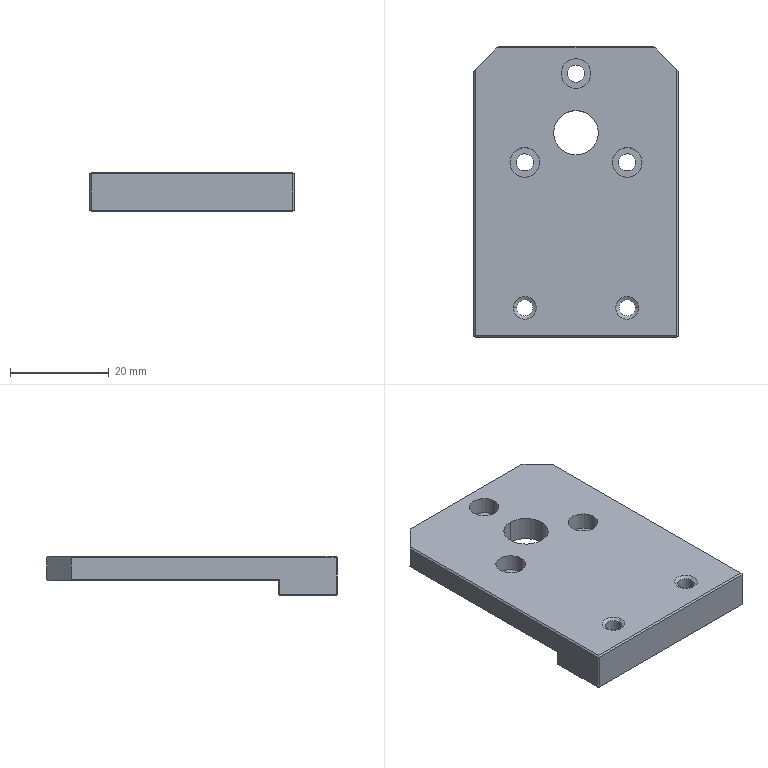Part | NX | 1 solid | 50 faces | box 41.5 x 59 x 8 mm | volume 12794 mm3 | plane 28 | cylinder 18 | cone 4 | commonest cylinder face diameters 3.5 x6 6 x6 3.3 x4 9 x2
STEP:
#1=CARTESIAN_POINT('',(-90.5,196.4,-40.777));
#2=VERTEX_POINT('',#1);
#3=CARTESIAN_POINT('',(-90.5,196.4,-43.777));
#4=VERTEX_POINT('',#3);
#5=CARTESIAN_POINT('',(-90.5,196.4,-42.427));
#6=DIRECTION('',(0.,0.,-1.));
#7=VECTOR('',#6,1000.);
#8=LINE('',#5,#7);
#9=EDGE_CURVE('',#2,#4,#8,.T.);
#10=ORIENTED_EDGE('',*,*,#9,.F.);
#11=CARTESIAN_POINT('',(-90.5,238.7,-40.777));
#12=VERTEX_POINT('',#11);
#13=CARTESIAN_POINT('',(-90.5,217.7,-40.777));
#14=DIRECTION('',(0.,-1.,0.));
#15=VECTOR('',#14,1000.);
#16=LINE('',#13,#15);
#17=EDGE_CURVE('',#12,#2,#16,.T.);
#18=ORIENTED_EDGE('',*,*,#17,.F.);
#19=CARTESIAN_POINT('',(-90.5,238.7,-36.377));
#20=VERTEX_POINT('',#19);
#21=CARTESIAN_POINT('',(-90.5,238.7,-38.577));
#22=DIRECTION('',(0.,0.,-1.));
#23=VECTOR('',#22,1000.);
#24=LINE('',#21,#23);
#25=EDGE_CURVE('',#20,#12,#24,.T.);
#26=ORIENTED_EDGE('',*,*,#25,.F.);
#27=CARTESIAN_POINT('',(-90.5,185.,-36.377));
#28=VERTEX_POINT('',#27);
#29=CARTESIAN_POINT('',(-90.5,211.7,-36.377));
#30=DIRECTION('',(0.,1.,0.));
#31=VECTOR('',#30,1000.);
#32=LINE('',#29,#31);
#33=EDGE_CURVE('',#28,#20,#32,.T.);
#34=ORIENTED_EDGE('',*,*,#33,.F.);
#35=CARTESIAN_POINT('',(-90.5,185.,-43.777));
#36=VERTEX_POINT('',#35);
#37=CARTESIAN_POINT('',(-90.5,185.,-40.077));
#38=DIRECTION('',(0.,0.,-1.));
#39=VECTOR('',#38,1000.);
#40=LINE('',#37,#39);
#41=EDGE_CURVE('',#28,#36,#40,.T.);
#42=ORIENTED_EDGE('',*,*,#41,.T.);
#43=CARTESIAN_POINT('',(-90.5,190.7,-43.777));
#44=DIRECTION('',(0.,-1.,0.));
#45=VECTOR('',#44,1000.);
#46=LINE('',#43,#45);
#47=EDGE_CURVE('',#4,#36,#46,.T.);
#48=ORIENTED_EDGE('',*,*,#47,.F.);
#49=EDGE_LOOP('',(#10,#18,#26,#34,#42,#48));
#50=FACE_BOUND('',#49,.T.);
#51=CARTESIAN_POINT('',(-90.5,208.7,-40.863));
#52=DIRECTION('',(1.,0.,0.));
#53=DIRECTION('',(0.,-1.,0.));
#54=AXIS2_PLACEMENT_3D('',#51,#52,#53);
#55=PLANE('',#54);
#56=ADVANCED_FACE('',(#50),#55,.T.);
#57=CARTESIAN_POINT('',(-131.7,185.,-36.077));
#58=VERTEX_POINT('',#57);
#59=CARTESIAN_POINT('',(-131.7,239.,-36.077));
#60=VERTEX_POINT('',#59);
#61=CARTESIAN_POINT('',(-131.7,0.,-36.077));
#62=DIRECTION('',(0.,1.,0.));
#63=VECTOR('',#62,1000.);
#64=LINE('',#61,#63);
#65=EDGE_CURVE('',#58,#60,#64,.T.);
#66=ORIENTED_EDGE('',*,*,#65,.F.);
#67=CARTESIAN_POINT('',(-90.8,185.,-36.077));
#68=VERTEX_POINT('',#67);
#69=CARTESIAN_POINT('',(0.,185.,-36.077));
#70=DIRECTION('',(1.,0.,0.));
#71=VECTOR('',#70,1000.);
#72=LINE('',#69,#71);
#73=EDGE_CURVE('',#58,#68,#72,.T.);
#74=ORIENTED_EDGE('',*,*,#73,.T.);
#75=CARTESIAN_POINT('',(-90.8,239.,-36.077));
#76=VERTEX_POINT('',#75);
#77=CARTESIAN_POINT('',(-90.8,0.,-36.077));
#78=DIRECTION('',(0.,1.,0.));
#79=VECTOR('',#78,1000.);
#80=LINE('',#77,#79);
#81=EDGE_CURVE('',#68,#76,#80,.T.);
#82=ORIENTED_EDGE('',*,*,#81,.T.);
#83=CARTESIAN_POINT('',(-95.2,243.4,-36.077));
#84=VERTEX_POINT('',#83);
#85=CARTESIAN_POINT('',(148.2,0.,-36.077));
#86=DIRECTION('',(0.7071,-0.7071,0.));
#87=VECTOR('',#86,1000.);
#88=LINE('',#85,#87);
#89=EDGE_CURVE('',#84,#76,#88,.T.);
#90=ORIENTED_EDGE('',*,*,#89,.F.);
#91=CARTESIAN_POINT('',(-127.3,243.4,-36.077));
#92=VERTEX_POINT('',#91);
#93=CARTESIAN_POINT('',(0.,243.4,-36.077));
#94=DIRECTION('',(-1.,0.,0.));
#95=VECTOR('',#94,1000.);
#96=LINE('',#93,#95);
#97=EDGE_CURVE('',#84,#92,#96,.T.);
#98=ORIENTED_EDGE('',*,*,#97,.T.);
#99=CARTESIAN_POINT('',(0.,370.7,-36.077));
#100=DIRECTION('',(0.7071,0.7071,0.));
#101=VECTOR('',#100,1000.);
#102=LINE('',#99,#101);
#103=EDGE_CURVE('',#60,#92,#102,.T.);
#104=ORIENTED_EDGE('',*,*,#103,.F.);
#105=EDGE_LOOP('',(#66,#74,#82,#90,#98,#104));
#106=FACE_BOUND('',#105,.T.);
#107=CARTESIAN_POINT('',(-114.25,238.2,-36.077));
#108=VERTEX_POINT('',#107);
#109=CARTESIAN_POINT('',(-108.25,238.2,-36.077));
#110=VERTEX_POINT('',#109);
#111=CARTESIAN_POINT('',(-111.25,238.2,-36.077));
#112=DIRECTION('',(0.,0.,1.));
#113=DIRECTION('',(-1.,0.,0.));
#114=AXIS2_PLACEMENT_3D('',#111,#112,#113);
#115=CIRCLE('',#114,3.);
#116=EDGE_CURVE('',#108,#110,#115,.T.);
#117=ORIENTED_EDGE('',*,*,#116,.F.);
#118=CARTESIAN_POINT('',(-111.25,238.2,-36.077));
#119=DIRECTION('',(0.,0.,1.));
#120=DIRECTION('',(-1.,0.,0.));
#121=AXIS2_PLACEMENT_3D('',#118,#119,#120);
#122=CIRCLE('',#121,3.);
#123=EDGE_CURVE('',#110,#108,#122,.T.);
#124=ORIENTED_EDGE('',*,*,#123,.F.);
#125=EDGE_LOOP('',(#117,#124));
#126=FACE_BOUND('',#125,.T.);
#127=CARTESIAN_POINT('',(-123.94,190.7,-36.077));
#128=VERTEX_POINT('',#127);
#129=CARTESIAN_POINT('',(-119.31,190.7,-36.077));
#130=VERTEX_POINT('',#129);
#131=CARTESIAN_POINT('',(-121.625,190.7,-36.077));
#132=DIRECTION('',(0.,0.,1.));
#133=DIRECTION('',(1.,0.,0.));
#134=AXIS2_PLACEMENT_3D('',#131,#132,#133);
#135=CIRCLE('',#134,2.315);
#136=EDGE_CURVE('',#128,#130,#135,.T.);
#137=ORIENTED_EDGE('',*,*,#136,.F.);
#138=CARTESIAN_POINT('',(-121.625,190.7,-36.077));
#139=DIRECTION('',(0.,0.,1.));
#140=DIRECTION('',(1.,0.,0.));
#141=AXIS2_PLACEMENT_3D('',#138,#139,#140);
#142=CIRCLE('',#141,2.315);
#143=EDGE_CURVE('',#130,#128,#142,.T.);
#144=ORIENTED_EDGE('',*,*,#143,.F.);
#145=EDGE_LOOP('',(#137,#144));
#146=FACE_BOUND('',#145,.T.);
#147=CARTESIAN_POINT('',(-118.642,220.2,-36.077));
#148=VERTEX_POINT('',#147);
#149=CARTESIAN_POINT('',(-124.642,220.2,-36.077));
#150=VERTEX_POINT('',#149);
#151=CARTESIAN_POINT('',(-121.642,220.2,-36.077));
#152=DIRECTION('',(0.,0.,1.));
#153=DIRECTION('',(-1.,0.,0.));
#154=AXIS2_PLACEMENT_3D('',#151,#152,#153);
#155=CIRCLE('',#154,3.);
#156=EDGE_CURVE('',#148,#150,#155,.T.);
#157=ORIENTED_EDGE('',*,*,#156,.F.);
#158=CARTESIAN_POINT('',(-121.642,220.2,-36.077));
#159=DIRECTION('',(0.,0.,1.));
#160=DIRECTION('',(-1.,0.,0.));
#161=AXIS2_PLACEMENT_3D('',#158,#159,#160);
#162=CIRCLE('',#161,3.);
#163=EDGE_CURVE('',#150,#148,#162,.T.);
#164=ORIENTED_EDGE('',*,*,#163,.F.);
#165=EDGE_LOOP('',(#157,#164));
#166=FACE_BOUND('',#165,.T.);
#167=CARTESIAN_POINT('',(-111.25,230.7,-36.077));
#168=VERTEX_POINT('',#167);
#169=CARTESIAN_POINT('',(-111.25,221.7,-36.077));
#170=VERTEX_POINT('',#169);
#171=CARTESIAN_POINT('',(-111.25,226.2,-36.077));
#172=DIRECTION('',(0.,0.,-1.));
#173=DIRECTION('',(0.,-1.,0.));
#174=AXIS2_PLACEMENT_3D('',#171,#172,#173);
#175=CIRCLE('',#174,4.5);
#176=EDGE_CURVE('',#168,#170,#175,.T.);
#177=ORIENTED_EDGE('',*,*,#176,.T.);
#178=CARTESIAN_POINT('',(-111.25,226.2,-36.077));
#179=DIRECTION('',(0.,0.,-1.));
#180=DIRECTION('',(0.,-1.,0.));
#181=AXIS2_PLACEMENT_3D('',#178,#179,#180);
#182=CIRCLE('',#181,4.5);
#183=EDGE_CURVE('',#170,#168,#182,.T.);
#184=ORIENTED_EDGE('',*,*,#183,.T.);
#185=EDGE_LOOP('',(#177,#184));
#186=FACE_BOUND('',#185,.T.);
#187=CARTESIAN_POINT('',(-97.858,220.2,-36.077));
#188=VERTEX_POINT('',#187);
#189=CARTESIAN_POINT('',(-103.858,220.2,-36.077));
#190=VERTEX_POINT('',#189);
#191=CARTESIAN_POINT('',(-100.858,220.2,-36.077));
#192=DIRECTION('',(0.,0.,1.));
#193=DIRECTION('',(-1.,0.,0.));
#194=AXIS2_PLACEMENT_3D('',#191,#192,#193);
#195=CIRCLE('',#194,3.);
#196=EDGE_CURVE('',#188,#190,#195,.T.);
#197=ORIENTED_EDGE('',*,*,#196,.F.);
#198=CARTESIAN_POINT('',(-100.858,220.2,-36.077));
#199=DIRECTION('',(0.,0.,1.));
#200=DIRECTION('',(-1.,0.,0.));
#201=AXIS2_PLACEMENT_3D('',#198,#199,#200);
#202=CIRCLE('',#201,3.);
#203=EDGE_CURVE('',#190,#188,#202,.T.);
#204=ORIENTED_EDGE('',*,*,#203,.F.);
#205=EDGE_LOOP('',(#197,#204));
#206=FACE_BOUND('',#205,.T.);
#207=CARTESIAN_POINT('',(-103.19,190.7,-36.077));
#208=VERTEX_POINT('',#207);
#209=CARTESIAN_POINT('',(-98.56,190.7,-36.077));
#210=VERTEX_POINT('',#209);
#211=CARTESIAN_POINT('',(-100.875,190.7,-36.077));
#212=DIRECTION('',(0.,0.,1.));
#213=DIRECTION('',(1.,0.,0.));
#214=AXIS2_PLACEMENT_3D('',#211,#212,#213);
#215=CIRCLE('',#214,2.315);
#216=EDGE_CURVE('',#208,#210,#215,.T.);
#217=ORIENTED_EDGE('',*,*,#216,.F.);
#218=CARTESIAN_POINT('',(-100.875,190.7,-36.077));
#219=DIRECTION('',(0.,0.,1.));
#220=DIRECTION('',(1.,0.,0.));
#221=AXIS2_PLACEMENT_3D('',#218,#219,#220);
#222=CIRCLE('',#221,2.315);
#223=EDGE_CURVE('',#210,#208,#222,.T.);
#224=ORIENTED_EDGE('',*,*,#223,.F.);
#225=EDGE_LOOP('',(#217,#224));
#226=FACE_BOUND('',#225,.T.);
#227=CARTESIAN_POINT('',(-137.,208.7,-36.077));
#228=DIRECTION('',(0.,0.,1.));
#229=DIRECTION('',(1.,0.,0.));
#230=AXIS2_PLACEMENT_3D('',#227,#228,#229);
#231=PLANE('',#230);
#232=ADVANCED_FACE('',(#106,#126,#146,#166,#186,#206,#226),#231,.T.);
#233=CARTESIAN_POINT('',(-132.,196.4,-43.777));
#234=VERTEX_POINT('',#233);
#235=CARTESIAN_POINT('',(-132.,196.4,-40.777));
#236=VERTEX_POINT('',#235);
#237=CARTESIAN_POINT('',(-132.,196.4,-42.427));
#238=DIRECTION('',(0.,0.,1.));
#239=VECTOR('',#238,1000.);
#240=LINE('',#237,#239);
#241=EDGE_CURVE('',#234,#236,#240,.T.);
#242=ORIENTED_EDGE('',*,*,#241,.F.);
#243=CARTESIAN_POINT('',(-132.,185.,-43.777));
#244=VERTEX_POINT('',#243);
#245=CARTESIAN_POINT('',(-132.,190.7,-43.777));
#246=DIRECTION('',(0.,1.,0.));
#247=VECTOR('',#246,1000.);
#248=LINE('',#245,#247);
#249=EDGE_CURVE('',#244,#234,#248,.T.);
#250=ORIENTED_EDGE('',*,*,#249,.F.);
#251=CARTESIAN_POINT('',(-132.,185.,-36.377));
#252=VERTEX_POINT('',#251);
#253=CARTESIAN_POINT('',(-132.,185.,-40.077));
#254=DIRECTION('',(0.,0.,1.));
#255=VECTOR('',#254,1000.);
#256=LINE('',#253,#255);
#257=EDGE_CURVE('',#244,#252,#256,.T.);
#258=ORIENTED_EDGE('',*,*,#257,.T.);
#259=CARTESIAN_POINT('',(-132.,238.7,-36.377));
#260=VERTEX_POINT('',#259);
#261=CARTESIAN_POINT('',(-132.,211.7,-36.377));
#262=DIRECTION('',(0.,-1.,0.));
#263=VECTOR('',#262,1000.);
#264=LINE('',#261,#263);
#265=EDGE_CURVE('',#260,#252,#264,.T.);
#266=ORIENTED_EDGE('',*,*,#265,.F.);
#267=CARTESIAN_POINT('',(-132.,238.7,-40.777));
#268=VERTEX_POINT('',#267);
#269=CARTESIAN_POINT('',(-132.,238.7,-38.577));
#270=DIRECTION('',(0.,0.,1.));
#271=VECTOR('',#270,1000.);
#272=LINE('',#269,#271);
#273=EDGE_CURVE('',#268,#260,#272,.T.);
#274=ORIENTED_EDGE('',*,*,#273,.F.);
#275=CARTESIAN_POINT('',(-132.,217.7,-40.777));
#276=DIRECTION('',(0.,1.,0.));
#277=VECTOR('',#276,1000.);
#278=LINE('',#275,#277);
#279=EDGE_CURVE('',#236,#268,#278,.T.);
#280=ORIENTED_EDGE('',*,*,#279,.F.);
#281=EDGE_LOOP('',(#242,#250,#258,#266,#274,#280));
#282=FACE_BOUND('',#281,.T.);
#283=CARTESIAN_POINT('',(-132.,208.7,-44.077));
#284=DIRECTION('',(-1.,0.,0.));
#285=DIRECTION('',(0.,0.,1.));
#286=AXIS2_PLACEMENT_3D('',#283,#284,#285);
#287=PLANE('',#286);
#288=ADVANCED_FACE('',(#282),#287,.T.);
#289=CARTESIAN_POINT('',(-127.3,243.4,-41.077));
#290=VERTEX_POINT('',#289);
#291=CARTESIAN_POINT('',(-95.2,243.4,-41.077));
#292=VERTEX_POINT('',#291);
#293=CARTESIAN_POINT('',(-111.25,243.4,-41.077));
#294=DIRECTION('',(1.,0.,0.));
#295=VECTOR('',#294,1000.);
#296=LINE('',#293,#295);
#297=EDGE_CURVE('',#290,#292,#296,.T.);
#298=ORIENTED_EDGE('',*,*,#297,.T.);
#299=CARTESIAN_POINT('',(-90.8,239.,-41.077));
#300=VERTEX_POINT('',#299);
#301=CARTESIAN_POINT('',(-60.5,208.7,-41.077));
#302=DIRECTION('',(-0.7071,0.7071,0.));
#303=VECTOR('',#302,1000.);
#304=LINE('',#301,#303);
#305=EDGE_CURVE('',#300,#292,#304,.T.);
#306=ORIENTED_EDGE('',*,*,#305,.F.);
#307=CARTESIAN_POINT('',(-90.8,196.7,-41.077));
#308=VERTEX_POINT('',#307);
#309=CARTESIAN_POINT('',(-90.8,217.7,-41.077));
#310=DIRECTION('',(0.,-1.,0.));
#311=VECTOR('',#310,1000.);
#312=LINE('',#309,#311);
#313=EDGE_CURVE('',#300,#308,#312,.T.);
#314=ORIENTED_EDGE('',*,*,#313,.T.);
#315=CARTESIAN_POINT('',(-131.7,196.7,-41.077));
#316=VERTEX_POINT('',#315);
#317=CARTESIAN_POINT('',(-128.319,196.7,-41.077));
#318=DIRECTION('',(1.,0.,0.));
#319=VECTOR('',#318,1000.);
#320=LINE('',#317,#319);
#321=EDGE_CURVE('',#316,#308,#320,.T.);
#322=ORIENTED_EDGE('',*,*,#321,.F.);
#323=CARTESIAN_POINT('',(-131.7,239.,-41.077));
#324=VERTEX_POINT('',#323);
#325=CARTESIAN_POINT('',(-131.7,217.7,-41.077));
#326=DIRECTION('',(0.,1.,0.));
#327=VECTOR('',#326,1000.);
#328=LINE('',#325,#327);
#329=EDGE_CURVE('',#316,#324,#328,.T.);
#330=ORIENTED_EDGE('',*,*,#329,.T.);
#331=CARTESIAN_POINT('',(-162.,208.7,-41.077));
#332=DIRECTION('',(-0.7071,-0.7071,0.));
#333=VECTOR('',#332,1000.);
#334=LINE('',#331,#333);
#335=EDGE_CURVE('',#290,#324,#334,.T.);
#336=ORIENTED_EDGE('',*,*,#335,.F.);
#337=EDGE_LOOP('',(#298,#306,#314,#322,#330,#336));
#338=FACE_BOUND('',#337,.T.);
#339=CARTESIAN_POINT('',(-111.25,230.7,-41.077));
#340=VERTEX_POINT('',#339);
#341=CARTESIAN_POINT('',(-111.25,221.7,-41.077));
#342=VERTEX_POINT('',#341);
#343=CARTESIAN_POINT('',(-111.25,226.2,-41.077));
#344=DIRECTION('',(0.,0.,-1.));
#345=DIRECTION('',(0.,-1.,0.));
#346=AXIS2_PLACEMENT_3D('',#343,#344,#345);
#347=CIRCLE('',#346,4.5);
#348=EDGE_CURVE('',#340,#342,#347,.T.);
#349=ORIENTED_EDGE('',*,*,#348,.F.);
#350=CARTESIAN_POINT('',(-111.25,226.2,-41.077));
#351=DIRECTION('',(0.,0.,-1.));
#352=DIRECTION('',(0.,-1.,0.));
#353=AXIS2_PLACEMENT_3D('',#350,#351,#352);
#354=CIRCLE('',#353,4.5);
#355=EDGE_CURVE('',#342,#340,#354,.T.);
#356=ORIENTED_EDGE('',*,*,#355,.F.);
#357=EDGE_LOOP('',(#349,#356));
#358=FACE_BOUND('',#357,.T.);
#359=CARTESIAN_POINT('',(-123.392,220.2,-41.077));
#360=VERTEX_POINT('',#359);
#361=CARTESIAN_POINT('',(-119.892,220.2,-41.077));
#362=VERTEX_POINT('',#361);
#363=CARTESIAN_POINT('',(-121.642,220.2,-41.077));
#364=DIRECTION('',(0.,0.,1.));
#365=DIRECTION('',(-1.,0.,0.));
#366=AXIS2_PLACEMENT_3D('',#363,#364,#365);
#367=CIRCLE('',#366,1.75);
#368=EDGE_CURVE('',#360,#362,#367,.T.);
#369=ORIENTED_EDGE('',*,*,#368,.T.);
#370=CARTESIAN_POINT('',(-121.642,220.2,-41.077));
#371=DIRECTION('',(0.,0.,1.));
#372=DIRECTION('',(-1.,0.,0.));
#373=AXIS2_PLACEMENT_3D('',#370,#371,#372);
#374=CIRCLE('',#373,1.75);
#375=EDGE_CURVE('',#362,#360,#374,.T.);
#376=ORIENTED_EDGE('',*,*,#375,.T.);
#377=EDGE_LOOP('',(#369,#376));
#378=FACE_BOUND('',#377,.T.);
#379=CARTESIAN_POINT('',(-113.,238.2,-41.077));
#380=VERTEX_POINT('',#379);
#381=CARTESIAN_POINT('',(-109.5,238.2,-41.077));
#382=VERTEX_POINT('',#381);
#383=CARTESIAN_POINT('',(-111.25,238.2,-41.077));
#384=DIRECTION('',(0.,0.,1.));
#385=DIRECTION('',(-1.,0.,0.));
#386=AXIS2_PLACEMENT_3D('',#383,#384,#385);
#387=CIRCLE('',#386,1.75);
#388=EDGE_CURVE('',#380,#382,#387,.T.);
#389=ORIENTED_EDGE('',*,*,#388,.T.);
#390=CARTESIAN_POINT('',(-111.25,238.2,-41.077));
#391=DIRECTION('',(0.,0.,1.));
#392=DIRECTION('',(-1.,0.,0.));
#393=AXIS2_PLACEMENT_3D('',#390,#391,#392);
#394=CIRCLE('',#393,1.75);
#395=EDGE_CURVE('',#382,#380,#394,.T.);
#396=ORIENTED_EDGE('',*,*,#395,.T.);
#397=EDGE_LOOP('',(#389,#396));
#398=FACE_BOUND('',#397,.T.);
#399=CARTESIAN_POINT('',(-99.108,220.2,-41.077));
#400=VERTEX_POINT('',#399);
#401=CARTESIAN_POINT('',(-102.608,220.2,-41.077));
#402=VERTEX_POINT('',#401);
#403=CARTESIAN_POINT('',(-100.858,220.2,-41.077));
#404=DIRECTION('',(0.,0.,1.));
#405=DIRECTION('',(-1.,0.,0.));
#406=AXIS2_PLACEMENT_3D('',#403,#404,#405);
#407=CIRCLE('',#406,1.75);
#408=EDGE_CURVE('',#400,#402,#407,.T.);
#409=ORIENTED_EDGE('',*,*,#408,.T.);
#410=CARTESIAN_POINT('',(-100.858,220.2,-41.077));
#411=DIRECTION('',(0.,0.,1.));
#412=DIRECTION('',(-1.,0.,0.));
#413=AXIS2_PLACEMENT_3D('',#410,#411,#412);
#414=CIRCLE('',#413,1.75);
#415=EDGE_CURVE('',#402,#400,#414,.T.);
#416=ORIENTED_EDGE('',*,*,#415,.T.);
#417=EDGE_LOOP('',(#409,#416));
#418=FACE_BOUND('',#417,.T.);
#419=CARTESIAN_POINT('',(-122.,208.7,-41.077));
#420=DIRECTION('',(0.,0.,-1.));
#421=DIRECTION('',(0.,-1.,0.));
#422=AXIS2_PLACEMENT_3D('',#419,#420,#421);
#423=PLANE('',#422);
#424=ADVANCED_FACE('',(#338,#358,#378,#398,#418),#423,.T.);
#425=ORIENTED_EDGE('',*,*,#321,.T.);
#426=CARTESIAN_POINT('',(-90.8,196.7,-43.777));
#427=VERTEX_POINT('',#426);
#428=CARTESIAN_POINT('',(-90.8,196.7,-42.427));
#429=DIRECTION('',(0.,0.,-1.));
#430=VECTOR('',#429,1000.);
#431=LINE('',#428,#430);
#432=EDGE_CURVE('',#308,#427,#431,.T.);
#433=ORIENTED_EDGE('',*,*,#432,.T.);
#434=CARTESIAN_POINT('',(-131.7,196.7,-43.777));
#435=VERTEX_POINT('',#434);
#436=CARTESIAN_POINT('',(-111.25,196.7,-43.777));
#437=DIRECTION('',(-1.,0.,0.));
#438=VECTOR('',#437,1000.);
#439=LINE('',#436,#438);
#440=EDGE_CURVE('',#427,#435,#439,.T.);
#441=ORIENTED_EDGE('',*,*,#440,.T.);
#442=CARTESIAN_POINT('',(-131.7,196.7,-42.427));
#443=DIRECTION('',(0.,0.,1.));
#444=VECTOR('',#443,1000.);
#445=LINE('',#442,#444);
#446=EDGE_CURVE('',#435,#316,#445,.T.);
#447=ORIENTED_EDGE('',*,*,#446,.T.);
#448=EDGE_LOOP('',(#425,#433,#441,#447));
#449=FACE_BOUND('',#448,.T.);
#450=CARTESIAN_POINT('',(-85.5,196.7,-41.077));
#451=DIRECTION('',(0.,1.,0.));
#452=DIRECTION('',(1.,0.,0.));
#453=AXIS2_PLACEMENT_3D('',#450,#451,#452);
#454=PLANE('',#453);
#455=ADVANCED_FACE('',(#449),#454,.T.);
#456=CARTESIAN_POINT('',(-90.8,185.,-44.077));
#457=VERTEX_POINT('',#456);
#458=CARTESIAN_POINT('',(-90.8,196.4,-44.077));
#459=VERTEX_POINT('',#458);
#460=CARTESIAN_POINT('',(-90.8,0.,-44.077));
#461=DIRECTION('',(0.,1.,0.));
#462=VECTOR('',#461,1000.);
#463=LINE('',#460,#462);
#464=EDGE_CURVE('',#457,#459,#463,.T.);
#465=ORIENTED_EDGE('',*,*,#464,.F.);
#466=CARTESIAN_POINT('',(-131.7,185.,-44.077));
#467=VERTEX_POINT('',#466);
#468=CARTESIAN_POINT('',(0.,185.,-44.077));
#469=DIRECTION('',(-1.,0.,0.));
#470=VECTOR('',#469,1000.);
#471=LINE('',#468,#470);
#472=EDGE_CURVE('',#457,#467,#471,.T.);
#473=ORIENTED_EDGE('',*,*,#472,.T.);
#474=CARTESIAN_POINT('',(-131.7,196.4,-44.077));
#475=VERTEX_POINT('',#474);
#476=CARTESIAN_POINT('',(-131.7,0.,-44.077));
#477=DIRECTION('',(0.,-1.,0.));
#478=VECTOR('',#477,1000.);
#479=LINE('',#476,#478);
#480=EDGE_CURVE('',#475,#467,#479,.T.);
#481=ORIENTED_EDGE('',*,*,#480,.F.);
#482=CARTESIAN_POINT('',(0.,196.4,-44.077));
#483=DIRECTION('',(1.,0.,0.));
#484=VECTOR('',#483,1000.);
#485=LINE('',#482,#484);
#486=EDGE_CURVE('',#475,#459,#485,.T.);
#487=ORIENTED_EDGE('',*,*,#486,.T.);
#488=EDGE_LOOP('',(#465,#473,#481,#487));
#489=FACE_BOUND('',#488,.T.);
#490=CARTESIAN_POINT('',(-102.525,190.7,-44.077));
#491=VERTEX_POINT('',#490);
#492=CARTESIAN_POINT('',(-99.225,190.7,-44.077));
#493=VERTEX_POINT('',#492);
#494=CARTESIAN_POINT('',(-100.875,190.7,-44.077));
#495=DIRECTION('',(0.,0.,1.));
#496=DIRECTION('',(1.,0.,0.));
#497=AXIS2_PLACEMENT_3D('',#494,#495,#496);
#498=CIRCLE('',#497,1.65);
#499=EDGE_CURVE('',#491,#493,#498,.T.);
#500=ORIENTED_EDGE('',*,*,#499,.T.);
#501=CARTESIAN_POINT('',(-100.875,190.7,-44.077));
#502=DIRECTION('',(0.,0.,1.));
#503=DIRECTION('',(1.,0.,0.));
#504=AXIS2_PLACEMENT_3D('',#501,#502,#503);
#505=CIRCLE('',#504,1.65);
#506=EDGE_CURVE('',#493,#491,#505,.T.);
#507=ORIENTED_EDGE('',*,*,#506,.T.);
#508=EDGE_LOOP('',(#500,#507));
#509=FACE_BOUND('',#508,.T.);
#510=CARTESIAN_POINT('',(-123.275,190.7,-44.077));
#511=VERTEX_POINT('',#510);
#512=CARTESIAN_POINT('',(-119.975,190.7,-44.077));
#513=VERTEX_POINT('',#512);
#514=CARTESIAN_POINT('',(-121.625,190.7,-44.077));
#515=DIRECTION('',(0.,0.,1.));
#516=DIRECTION('',(1.,0.,0.));
#517=AXIS2_PLACEMENT_3D('',#514,#515,#516);
#518=CIRCLE('',#517,1.65);
#519=EDGE_CURVE('',#511,#513,#518,.T.);
#520=ORIENTED_EDGE('',*,*,#519,.T.);
#521=CARTESIAN_POINT('',(-121.625,190.7,-44.077));
#522=DIRECTION('',(0.,0.,1.));
#523=DIRECTION('',(1.,0.,0.));
#524=AXIS2_PLACEMENT_3D('',#521,#522,#523);
#525=CIRCLE('',#524,1.65);
#526=EDGE_CURVE('',#513,#511,#525,.T.);
#527=ORIENTED_EDGE('',*,*,#526,.T.);
#528=EDGE_LOOP('',(#520,#527));
#529=FACE_BOUND('',#528,.T.);
#530=CARTESIAN_POINT('',(-88.698,210.445,-44.077));
#531=DIRECTION('',(0.,0.,-1.));
#532=DIRECTION('',(0.,-1.,0.));
#533=AXIS2_PLACEMENT_3D('',#530,#531,#532);
#534=PLANE('',#533);
#535=ADVANCED_FACE('',(#489,#509,#529),#534,.T.);
#536=ORIENTED_EDGE('',*,*,#348,.T.);
#537=CARTESIAN_POINT('',(-111.25,221.7,-35.277));
#538=DIRECTION('',(0.,0.,-1.));
#539=VECTOR('',#538,1000.);
#540=LINE('',#537,#539);
#541=EDGE_CURVE('',#342,#170,#540,.F.);
#542=ORIENTED_EDGE('',*,*,#541,.T.);
#543=ORIENTED_EDGE('',*,*,#176,.F.);
#544=CARTESIAN_POINT('',(-111.25,230.7,-35.277));
#545=DIRECTION('',(0.,0.,-1.));
#546=VECTOR('',#545,1000.);
#547=LINE('',#544,#546);
#548=EDGE_CURVE('',#340,#168,#547,.F.);
#549=ORIENTED_EDGE('',*,*,#548,.F.);
#550=EDGE_LOOP('',(#536,#542,#543,#549));
#551=FACE_BOUND('',#550,.T.);
#552=CARTESIAN_POINT('',(-111.25,226.2,-35.277));
#553=DIRECTION('',(0.,0.,-1.));
#554=DIRECTION('',(0.,-1.,0.));
#555=AXIS2_PLACEMENT_3D('',#552,#553,#554);
#556=CYLINDRICAL_SURFACE('',#555,4.5);
#557=ADVANCED_FACE('',(#551),#556,.F.);
#558=ORIENTED_EDGE('',*,*,#464,.T.);
#559=CARTESIAN_POINT('',(-90.65,196.55,-43.927));
#560=VERTEX_POINT('',#559);
#561=CARTESIAN_POINT('',(-78.5,208.7,-31.777));
#562=DIRECTION('',(0.5774,0.5774,0.5774));
#563=VECTOR('',#562,1000.);
#564=LINE('',#561,#563);
#565=EDGE_CURVE('',#459,#560,#564,.T.);
#566=ORIENTED_EDGE('',*,*,#565,.T.);
#567=CARTESIAN_POINT('',(-89.502,195.402,-42.779));
#568=DIRECTION('',(0.5774,-0.5774,0.5774));
#569=VECTOR('',#568,1000.);
#570=LINE('',#567,#569);
#571=EDGE_CURVE('',#560,#4,#570,.T.);
#572=ORIENTED_EDGE('',*,*,#571,.T.);
#573=ORIENTED_EDGE('',*,*,#47,.T.);
#574=CARTESIAN_POINT('',(-90.65,184.85,-43.927));
#575=VERTEX_POINT('',#574);
#576=CARTESIAN_POINT('',(-66.8,208.7,-20.077));
#577=DIRECTION('',(0.5774,0.5774,0.5774));
#578=VECTOR('',#577,1000.);
#579=LINE('',#576,#578);
#580=EDGE_CURVE('',#575,#36,#579,.T.);
#581=ORIENTED_EDGE('',*,*,#580,.F.);
#582=CARTESIAN_POINT('',(-114.5,208.7,-67.777));
#583=DIRECTION('',(-0.5774,0.5774,-0.5774));
#584=VECTOR('',#583,1000.);
#585=LINE('',#582,#584);
#586=EDGE_CURVE('',#575,#457,#585,.T.);
#587=ORIENTED_EDGE('',*,*,#586,.T.);
#588=EDGE_LOOP('',(#558,#566,#572,#573,#581,#587));
#589=FACE_BOUND('',#588,.T.);
#590=CARTESIAN_POINT('',(-90.65,190.7,-43.927));
#591=DIRECTION('',(0.7071,0.,-0.7071));
#592=DIRECTION('',(0.,-1.,0.));
#593=AXIS2_PLACEMENT_3D('',#590,#591,#592);
#594=PLANE('',#593);
#595=ADVANCED_FACE('',(#589),#594,.T.);
#596=ORIENTED_EDGE('',*,*,#33,.T.);
#597=CARTESIAN_POINT('',(-84.098,232.298,-42.779));
#598=DIRECTION('',(0.5774,-0.5774,-0.5774));
#599=VECTOR('',#598,1000.);
#600=LINE('',#597,#599);
#601=EDGE_CURVE('',#76,#20,#600,.T.);
#602=ORIENTED_EDGE('',*,*,#601,.F.);
#603=ORIENTED_EDGE('',*,*,#81,.F.);
#604=CARTESIAN_POINT('',(-90.65,184.85,-36.227));
#605=VERTEX_POINT('',#604);
#606=CARTESIAN_POINT('',(-114.5,208.7,-12.377));
#607=DIRECTION('',(-0.5774,0.5774,0.5774));
#608=VECTOR('',#607,1000.);
#609=LINE('',#606,#608);
#610=EDGE_CURVE('',#605,#68,#609,.T.);
#611=ORIENTED_EDGE('',*,*,#610,.F.);
#612=CARTESIAN_POINT('',(-66.8,208.7,-60.077));
#613=DIRECTION('',(0.5774,0.5774,-0.5774));
#614=VECTOR('',#613,1000.);
#615=LINE('',#612,#614);
#616=EDGE_CURVE('',#605,#28,#615,.T.);
#617=ORIENTED_EDGE('',*,*,#616,.T.);
#618=EDGE_LOOP('',(#596,#602,#603,#611,#617));
#619=FACE_BOUND('',#618,.T.);
#620=CARTESIAN_POINT('',(-90.65,211.7,-36.227));
#621=DIRECTION('',(-0.7071,0.,-0.7071));
#622=DIRECTION('',(-0.7071,0.,0.7071));
#623=AXIS2_PLACEMENT_3D('',#620,#621,#622);
#624=PLANE('',#623);
#625=ADVANCED_FACE('',(#619),#624,.F.);
#626=ORIENTED_EDGE('',*,*,#472,.F.);
#627=ORIENTED_EDGE('',*,*,#586,.F.);
#628=CARTESIAN_POINT('',(-90.8,184.7,-43.777));
#629=VERTEX_POINT('',#628);
#630=CARTESIAN_POINT('',(-66.8,208.7,-67.777));
#631=DIRECTION('',(-0.5774,-0.5774,0.5774));
#632=VECTOR('',#631,1000.);
#633=LINE('',#630,#632);
#634=EDGE_CURVE('',#575,#629,#633,.T.);
#635=ORIENTED_EDGE('',*,*,#634,.T.);
#636=CARTESIAN_POINT('',(-131.7,184.7,-43.777));
#637=VERTEX_POINT('',#636);
#638=CARTESIAN_POINT('',(-111.25,184.7,-43.777));
#639=DIRECTION('',(1.,0.,0.));
#640=VECTOR('',#639,1000.);
#641=LINE('',#638,#640);
#642=EDGE_CURVE('',#637,#629,#641,.T.);
#643=ORIENTED_EDGE('',*,*,#642,.F.);
#644=CARTESIAN_POINT('',(-131.85,184.85,-43.927));
#645=VERTEX_POINT('',#644);
#646=CARTESIAN_POINT('',(-155.7,208.7,-67.777));
#647=DIRECTION('',(0.5774,-0.5774,0.5774));
#648=VECTOR('',#647,1000.);
#649=LINE('',#646,#648);
#650=EDGE_CURVE('',#645,#637,#649,.T.);
#651=ORIENTED_EDGE('',*,*,#650,.F.);
#652=CARTESIAN_POINT('',(-108.,208.7,-67.777));
#653=DIRECTION('',(0.5774,0.5774,-0.5774));
#654=VECTOR('',#653,1000.);
#655=LINE('',#652,#654);
#656=EDGE_CURVE('',#645,#467,#655,.T.);
#657=ORIENTED_EDGE('',*,*,#656,.T.);
#658=EDGE_LOOP('',(#626,#627,#635,#643,#651,#657));
#659=FACE_BOUND('',#658,.T.);
#660=CARTESIAN_POINT('',(-111.25,184.85,-43.927));
#661=DIRECTION('',(0.,0.7071,0.7071));
#662=DIRECTION('',(1.,0.,0.));
#663=AXIS2_PLACEMENT_3D('',#660,#661,#662);
#664=PLANE('',#663);
#665=ADVANCED_FACE('',(#659),#664,.F.);
#666=ORIENTED_EDGE('',*,*,#486,.F.);
#667=CARTESIAN_POINT('',(-131.85,196.55,-43.927));
#668=VERTEX_POINT('',#667);
#669=CARTESIAN_POINT('',(-132.998,197.698,-42.779));
#670=DIRECTION('',(-0.5774,0.5774,0.5774));
#671=VECTOR('',#670,1000.);
#672=LINE('',#669,#671);
#673=EDGE_CURVE('',#475,#668,#672,.T.);
#674=ORIENTED_EDGE('',*,*,#673,.T.);
#675=CARTESIAN_POINT('',(-119.7,208.7,-31.777));
#676=DIRECTION('',(-0.5774,-0.5774,-0.5774));
#677=VECTOR('',#676,1000.);
#678=LINE('',#675,#677);
#679=EDGE_CURVE('',#435,#668,#678,.T.);
#680=ORIENTED_EDGE('',*,*,#679,.F.);
#681=ORIENTED_EDGE('',*,*,#440,.F.);
#682=CARTESIAN_POINT('',(-91.798,197.698,-42.779));
#683=DIRECTION('',(-0.5774,0.5774,0.5774));
#684=VECTOR('',#683,1000.);
#685=LINE('',#682,#684);
#686=EDGE_CURVE('',#560,#427,#685,.T.);
#687=ORIENTED_EDGE('',*,*,#686,.F.);
#688=ORIENTED_EDGE('',*,*,#565,.F.);
#689=EDGE_LOOP('',(#666,#674,#680,#681,#687,#688));
#690=FACE_BOUND('',#689,.T.);
#691=CARTESIAN_POINT('',(-111.25,196.55,-43.927));
#692=DIRECTION('',(0.,-0.7071,0.7071));
#693=DIRECTION('',(-1.,0.,0.));
#694=AXIS2_PLACEMENT_3D('',#691,#692,#693);
#695=PLANE('',#694);
#696=ADVANCED_FACE('',(#690),#695,.F.);
#697=ORIENTED_EDGE('',*,*,#9,.T.);
#698=ORIENTED_EDGE('',*,*,#571,.F.);
#699=ORIENTED_EDGE('',*,*,#686,.T.);
#700=ORIENTED_EDGE('',*,*,#432,.F.);
#701=CARTESIAN_POINT('',(-92.502,198.402,-42.779));
#702=DIRECTION('',(0.5774,-0.5774,0.5774));
#703=VECTOR('',#702,1000.);
#704=LINE('',#701,#703);
#705=EDGE_CURVE('',#308,#2,#704,.T.);
#706=ORIENTED_EDGE('',*,*,#705,.T.);
#707=EDGE_LOOP('',(#697,#698,#699,#700,#706));
#708=FACE_BOUND('',#707,.T.);
#709=CARTESIAN_POINT('',(-90.65,196.55,-42.427));
#710=DIRECTION('',(-0.7071,-0.7071,0.));
#711=DIRECTION('',(-0.7071,0.7071,0.));
#712=AXIS2_PLACEMENT_3D('',#709,#710,#711);
#713=PLANE('',#712);
#714=ADVANCED_FACE('',(#708),#713,.F.);
#715=ORIENTED_EDGE('',*,*,#17,.T.);
#716=ORIENTED_EDGE('',*,*,#705,.F.);
#717=ORIENTED_EDGE('',*,*,#313,.F.);
#718=CARTESIAN_POINT('',(-92.502,240.702,-42.779));
#719=DIRECTION('',(-0.5774,0.5774,-0.5774));
#720=VECTOR('',#719,1000.);
#721=LINE('',#718,#720);
#722=EDGE_CURVE('',#12,#300,#721,.T.);
#723=ORIENTED_EDGE('',*,*,#722,.F.);
#724=EDGE_LOOP('',(#715,#716,#717,#723));
#725=FACE_BOUND('',#724,.T.);
#726=CARTESIAN_POINT('',(-90.65,217.7,-40.927));
#727=DIRECTION('',(-0.7071,0.,0.7071));
#728=DIRECTION('',(0.,1.,0.));
#729=AXIS2_PLACEMENT_3D('',#726,#727,#728);
#730=PLANE('',#729);
#731=ADVANCED_FACE('',(#725),#730,.F.);
#732=ORIENTED_EDGE('',*,*,#279,.T.);
#733=CARTESIAN_POINT('',(-162.,208.7,-10.777));
#734=DIRECTION('',(-0.5774,-0.5774,0.5774));
#735=VECTOR('',#734,1000.);
#736=LINE('',#733,#735);
#737=EDGE_CURVE('',#324,#268,#736,.T.);
#738=ORIENTED_EDGE('',*,*,#737,.F.);
#739=ORIENTED_EDGE('',*,*,#329,.F.);
#740=CARTESIAN_POINT('',(-119.7,208.7,-53.077));
#741=DIRECTION('',(0.5774,0.5774,-0.5774));
#742=VECTOR('',#741,1000.);
#743=LINE('',#740,#742);
#744=EDGE_CURVE('',#236,#316,#743,.T.);
#745=ORIENTED_EDGE('',*,*,#744,.F.);
#746=EDGE_LOOP('',(#732,#738,#739,#745));
#747=FACE_BOUND('',#746,.T.);
#748=CARTESIAN_POINT('',(-131.85,217.7,-40.927));
#749=DIRECTION('',(0.7071,0.,0.7071));
#750=DIRECTION('',(0.,-1.,0.));
#751=AXIS2_PLACEMENT_3D('',#748,#749,#750);
#752=PLANE('',#751);
#753=ADVANCED_FACE('',(#747),#752,.F.);
#754=ORIENTED_EDGE('',*,*,#241,.T.);
#755=ORIENTED_EDGE('',*,*,#744,.T.);
#756=ORIENTED_EDGE('',*,*,#446,.F.);
#757=ORIENTED_EDGE('',*,*,#679,.T.);
#758=CARTESIAN_POINT('',(-119.7,208.7,-56.077));
#759=DIRECTION('',(0.5774,0.5774,-0.5774));
#760=VECTOR('',#759,1000.);
#761=LINE('',#758,#760);
#762=EDGE_CURVE('',#234,#668,#761,.T.);
#763=ORIENTED_EDGE('',*,*,#762,.F.);
#764=EDGE_LOOP('',(#754,#755,#756,#757,#763));
#765=FACE_BOUND('',#764,.T.);
#766=CARTESIAN_POINT('',(-131.85,196.55,-42.427));
#767=DIRECTION('',(0.7071,-0.7071,0.));
#768=DIRECTION('',(0.,0.,-1.));
#769=AXIS2_PLACEMENT_3D('',#766,#767,#768);
#770=PLANE('',#769);
#771=ADVANCED_FACE('',(#765),#770,.F.);
#772=CARTESIAN_POINT('',(-95.5,243.7,-36.377));
#773=VERTEX_POINT('',#772);
#774=CARTESIAN_POINT('',(-95.5,243.7,-40.777));
#775=VERTEX_POINT('',#774);
#776=CARTESIAN_POINT('',(-95.5,243.7,-38.577));
#777=DIRECTION('',(0.,0.,-1.));
#778=VECTOR('',#777,1000.);
#779=LINE('',#776,#778);
#780=EDGE_CURVE('',#773,#775,#779,.T.);
#781=ORIENTED_EDGE('',*,*,#780,.F.);
#782=CARTESIAN_POINT('',(-101.902,250.102,-42.779));
#783=DIRECTION('',(0.5774,-0.5774,0.5774));
#784=VECTOR('',#783,1000.);
#785=LINE('',#782,#784);
#786=EDGE_CURVE('',#773,#84,#785,.T.);
#787=ORIENTED_EDGE('',*,*,#786,.T.);
#788=ORIENTED_EDGE('',*,*,#89,.T.);
#789=ORIENTED_EDGE('',*,*,#601,.T.);
#790=ORIENTED_EDGE('',*,*,#25,.T.);
#791=ORIENTED_EDGE('',*,*,#722,.T.);
#792=ORIENTED_EDGE('',*,*,#305,.T.);
#793=CARTESIAN_POINT('',(-93.498,241.698,-42.779));
#794=DIRECTION('',(-0.5774,0.5774,0.5774));
#795=VECTOR('',#794,1000.);
#796=LINE('',#793,#795);
#797=EDGE_CURVE('',#292,#775,#796,.T.);
#798=ORIENTED_EDGE('',*,*,#797,.T.);
#799=EDGE_LOOP('',(#781,#787,#788,#789,#790,#791,#792,#798));
#800=FACE_BOUND('',#799,.T.);
#801=CARTESIAN_POINT('',(-93.,241.2,-38.577));
#802=DIRECTION('',(0.7071,0.7071,0.));
#803=DIRECTION('',(0.,0.,-1.));
#804=AXIS2_PLACEMENT_3D('',#801,#802,#803);
#805=PLANE('',#804);
#806=ADVANCED_FACE('',(#800),#805,.T.);
#807=CARTESIAN_POINT('',(-131.7,184.7,-36.377));
#808=VERTEX_POINT('',#807);
#809=CARTESIAN_POINT('',(-90.8,184.7,-36.377));
#810=VERTEX_POINT('',#809);
#811=CARTESIAN_POINT('',(-111.25,184.7,-36.377));
#812=DIRECTION('',(1.,0.,0.));
#813=VECTOR('',#812,1000.);
#814=LINE('',#811,#813);
#815=EDGE_CURVE('',#808,#810,#814,.T.);
#816=ORIENTED_EDGE('',*,*,#815,.T.);
#817=CARTESIAN_POINT('',(-66.8,208.7,-12.377));
#818=DIRECTION('',(0.5774,0.5774,0.5774));
#819=VECTOR('',#818,1000.);
#820=LINE('',#817,#819);
#821=EDGE_CURVE('',#810,#605,#820,.T.);
#822=ORIENTED_EDGE('',*,*,#821,.T.);
#823=ORIENTED_EDGE('',*,*,#610,.T.);
#824=ORIENTED_EDGE('',*,*,#73,.F.);
#825=CARTESIAN_POINT('',(-131.85,184.85,-36.227));
#826=VERTEX_POINT('',#825);
#827=CARTESIAN_POINT('',(-108.,208.7,-12.377));
#828=DIRECTION('',(0.5774,0.5774,0.5774));
#829=VECTOR('',#828,1000.);
#830=LINE('',#827,#829);
#831=EDGE_CURVE('',#826,#58,#830,.T.);
#832=ORIENTED_EDGE('',*,*,#831,.F.);
#833=CARTESIAN_POINT('',(-155.7,208.7,-12.377));
#834=DIRECTION('',(0.5774,-0.5774,-0.5774));
#835=VECTOR('',#834,1000.);
#836=LINE('',#833,#835);
#837=EDGE_CURVE('',#826,#808,#836,.T.);
#838=ORIENTED_EDGE('',*,*,#837,.T.);
#839=EDGE_LOOP('',(#816,#822,#823,#824,#832,#838));
#840=FACE_BOUND('',#839,.T.);
#841=CARTESIAN_POINT('',(-111.25,184.85,-36.227));
#842=DIRECTION('',(0.,0.7071,-0.7071));
#843=DIRECTION('',(-1.,0.,0.));
#844=AXIS2_PLACEMENT_3D('',#841,#842,#843);
#845=PLANE('',#844);
#846=ADVANCED_FACE('',(#840),#845,.F.);
#847=ORIENTED_EDGE('',*,*,#65,.T.);
#848=CARTESIAN_POINT('',(-162.,208.7,-66.377));
#849=DIRECTION('',(-0.5774,-0.5774,-0.5774));
#850=VECTOR('',#849,1000.);
#851=LINE('',#848,#850);
#852=EDGE_CURVE('',#60,#260,#851,.T.);
#853=ORIENTED_EDGE('',*,*,#852,.T.);
#854=ORIENTED_EDGE('',*,*,#265,.T.);
#855=CARTESIAN_POINT('',(-155.7,208.7,-60.077));
#856=DIRECTION('',(0.5774,-0.5774,0.5774));
#857=VECTOR('',#856,1000.);
#858=LINE('',#855,#857);
#859=EDGE_CURVE('',#252,#826,#858,.T.);
#860=ORIENTED_EDGE('',*,*,#859,.T.);
#861=ORIENTED_EDGE('',*,*,#831,.T.);
#862=EDGE_LOOP('',(#847,#853,#854,#860,#861));
#863=FACE_BOUND('',#862,.T.);
#864=CARTESIAN_POINT('',(-131.85,211.7,-36.227));
#865=DIRECTION('',(-0.7071,0.,0.7071));
#866=DIRECTION('',(0.,1.,0.));
#867=AXIS2_PLACEMENT_3D('',#864,#865,#866);
#868=PLANE('',#867);
#869=ADVANCED_FACE('',(#863),#868,.T.);
#870=ORIENTED_EDGE('',*,*,#480,.T.);
#871=ORIENTED_EDGE('',*,*,#656,.F.);
#872=CARTESIAN_POINT('',(-132.998,185.998,-42.779));
#873=DIRECTION('',(-0.5774,0.5774,0.5774));
#874=VECTOR('',#873,1000.);
#875=LINE('',#872,#874);
#876=EDGE_CURVE('',#645,#244,#875,.T.);
#877=ORIENTED_EDGE('',*,*,#876,.T.);
#878=ORIENTED_EDGE('',*,*,#249,.T.);
#879=ORIENTED_EDGE('',*,*,#762,.T.);
#880=ORIENTED_EDGE('',*,*,#673,.F.);
#881=EDGE_LOOP('',(#870,#871,#877,#878,#879,#880));
#882=FACE_BOUND('',#881,.T.);
#883=CARTESIAN_POINT('',(-131.85,190.7,-43.927));
#884=DIRECTION('',(-0.7071,0.,-0.7071));
#885=DIRECTION('',(-0.7071,0.,0.7071));
#886=AXIS2_PLACEMENT_3D('',#883,#884,#885);
#887=PLANE('',#886);
#888=ADVANCED_FACE('',(#882),#887,.T.);
#889=ORIENTED_EDGE('',*,*,#368,.F.);
#890=CARTESIAN_POINT('',(-123.392,220.2,-39.577));
#891=VERTEX_POINT('',#890);
#892=CARTESIAN_POINT('',(-123.392,220.2,-36.077));
#893=DIRECTION('',(0.,0.,1.));
#894=VECTOR('',#893,1000.);
#895=LINE('',#892,#894);
#896=EDGE_CURVE('',#891,#360,#895,.F.);
#897=ORIENTED_EDGE('',*,*,#896,.F.);
#898=CARTESIAN_POINT('',(-119.892,220.2,-39.577));
#899=VERTEX_POINT('',#898);
#900=CARTESIAN_POINT('',(-121.642,220.2,-39.577));
#901=DIRECTION('',(0.,0.,1.));
#902=DIRECTION('',(-1.,0.,0.));
#903=AXIS2_PLACEMENT_3D('',#900,#901,#902);
#904=CIRCLE('',#903,1.75);
#905=EDGE_CURVE('',#891,#899,#904,.T.);
#906=ORIENTED_EDGE('',*,*,#905,.T.);
#907=CARTESIAN_POINT('',(-119.892,220.2,-36.077));
#908=DIRECTION('',(0.,0.,1.));
#909=VECTOR('',#908,1000.);
#910=LINE('',#907,#909);
#911=EDGE_CURVE('',#899,#362,#910,.F.);
#912=ORIENTED_EDGE('',*,*,#911,.T.);
#913=EDGE_LOOP('',(#889,#897,#906,#912));
#914=FACE_BOUND('',#913,.T.);
#915=CARTESIAN_POINT('',(-121.642,220.2,-36.077));
#916=DIRECTION('',(0.,0.,1.));
#917=DIRECTION('',(-1.,0.,0.));
#918=AXIS2_PLACEMENT_3D('',#915,#916,#917);
#919=CYLINDRICAL_SURFACE('',#918,1.75);
#920=ADVANCED_FACE('',(#914),#919,.F.);
#921=CARTESIAN_POINT('',(-124.642,220.2,-39.577));
#922=VERTEX_POINT('',#921);
#923=CARTESIAN_POINT('',(-118.642,220.2,-39.577));
#924=VERTEX_POINT('',#923);
#925=CARTESIAN_POINT('',(-121.642,220.2,-39.577));
#926=DIRECTION('',(0.,0.,1.));
#927=DIRECTION('',(-1.,0.,0.));
#928=AXIS2_PLACEMENT_3D('',#925,#926,#927);
#929=CIRCLE('',#928,3.);
#930=EDGE_CURVE('',#922,#924,#929,.T.);
#931=ORIENTED_EDGE('',*,*,#930,.T.);
#932=CARTESIAN_POINT('',(-121.642,220.2,-39.577));
#933=DIRECTION('',(0.,0.,1.));
#934=DIRECTION('',(-1.,0.,0.));
#935=AXIS2_PLACEMENT_3D('',#932,#933,#934);
#936=CIRCLE('',#935,3.);
#937=EDGE_CURVE('',#924,#922,#936,.T.);
#938=ORIENTED_EDGE('',*,*,#937,.T.);
#939=EDGE_LOOP('',(#931,#938));
#940=FACE_BOUND('',#939,.T.);
#941=ORIENTED_EDGE('',*,*,#905,.F.);
#942=CARTESIAN_POINT('',(-121.642,220.2,-39.577));
#943=DIRECTION('',(0.,0.,1.));
#944=DIRECTION('',(-1.,0.,0.));
#945=AXIS2_PLACEMENT_3D('',#942,#943,#944);
#946=CIRCLE('',#945,1.75);
#947=EDGE_CURVE('',#899,#891,#946,.T.);
#948=ORIENTED_EDGE('',*,*,#947,.F.);
#949=EDGE_LOOP('',(#941,#948));
#950=FACE_BOUND('',#949,.T.);
#951=CARTESIAN_POINT('',(-121.642,220.2,-39.577));
#952=DIRECTION('',(0.,0.,1.));
#953=DIRECTION('',(1.,0.,0.));
#954=AXIS2_PLACEMENT_3D('',#951,#952,#953);
#955=PLANE('',#954);
#956=ADVANCED_FACE('',(#940,#950),#955,.T.);
#957=ORIENTED_EDGE('',*,*,#930,.F.);
#958=CARTESIAN_POINT('',(-124.642,220.2,-36.077));
#959=DIRECTION('',(0.,0.,1.));
#960=VECTOR('',#959,1000.);
#961=LINE('',#958,#960);
#962=EDGE_CURVE('',#150,#922,#961,.F.);
#963=ORIENTED_EDGE('',*,*,#962,.F.);
#964=ORIENTED_EDGE('',*,*,#163,.T.);
#965=CARTESIAN_POINT('',(-118.642,220.2,-36.077));
#966=DIRECTION('',(0.,0.,1.));
#967=VECTOR('',#966,1000.);
#968=LINE('',#965,#967);
#969=EDGE_CURVE('',#148,#924,#968,.F.);
#970=ORIENTED_EDGE('',*,*,#969,.T.);
#971=EDGE_LOOP('',(#957,#963,#964,#970));
#972=FACE_BOUND('',#971,.T.);
#973=CARTESIAN_POINT('',(-121.642,220.2,-36.077));
#974=DIRECTION('',(0.,0.,1.));
#975=DIRECTION('',(-1.,0.,0.));
#976=AXIS2_PLACEMENT_3D('',#973,#974,#975);
#977=CYLINDRICAL_SURFACE('',#976,3.);
#978=ADVANCED_FACE('',(#972),#977,.F.);
#979=CARTESIAN_POINT('',(-113.,238.2,-39.577));
#980=VERTEX_POINT('',#979);
#981=CARTESIAN_POINT('',(-109.5,238.2,-39.577));
#982=VERTEX_POINT('',#981);
#983=CARTESIAN_POINT('',(-111.25,238.2,-39.577));
#984=DIRECTION('',(0.,0.,1.));
#985=DIRECTION('',(-1.,0.,0.));
#986=AXIS2_PLACEMENT_3D('',#983,#984,#985);
#987=CIRCLE('',#986,1.75);
#988=EDGE_CURVE('',#980,#982,#987,.T.);
#989=ORIENTED_EDGE('',*,*,#988,.T.);
#990=CARTESIAN_POINT('',(-109.5,238.2,-36.077));
#991=DIRECTION('',(0.,0.,1.));
#992=VECTOR('',#991,1000.);
#993=LINE('',#990,#992);
#994=EDGE_CURVE('',#982,#382,#993,.F.);
#995=ORIENTED_EDGE('',*,*,#994,.T.);
#996=ORIENTED_EDGE('',*,*,#388,.F.);
#997=CARTESIAN_POINT('',(-113.,238.2,-36.077));
#998=DIRECTION('',(0.,0.,1.));
#999=VECTOR('',#998,1000.);
#1000=LINE('',#997,#999);
#1001=EDGE_CURVE('',#980,#380,#1000,.F.);
#1002=ORIENTED_EDGE('',*,*,#1001,.F.);
#1003=EDGE_LOOP('',(#989,#995,#996,#1002));
#1004=FACE_BOUND('',#1003,.T.);
#1005=CARTESIAN_POINT('',(-111.25,238.2,-36.077));
#1006=DIRECTION('',(0.,0.,1.));
#1007=DIRECTION('',(-1.,0.,0.));
#1008=AXIS2_PLACEMENT_3D('',#1005,#1006,#1007);
#1009=CYLINDRICAL_SURFACE('',#1008,1.75);
#1010=ADVANCED_FACE('',(#1004),#1009,.F.);
#1011=CARTESIAN_POINT('',(-114.25,238.2,-39.577));
#1012=VERTEX_POINT('',#1011);
#1013=CARTESIAN_POINT('',(-108.25,238.2,-39.577));
#1014=VERTEX_POINT('',#1013);
#1015=CARTESIAN_POINT('',(-111.25,238.2,-39.577));
#1016=DIRECTION('',(0.,0.,1.));
#1017=DIRECTION('',(-1.,0.,0.));
#1018=AXIS2_PLACEMENT_3D('',#1015,#1016,#1017);
#1019=CIRCLE('',#1018,3.);
#1020=EDGE_CURVE('',#1012,#1014,#1019,.T.);
#1021=ORIENTED_EDGE('',*,*,#1020,.T.);
#1022=CARTESIAN_POINT('',(-111.25,238.2,-39.577));
#1023=DIRECTION('',(0.,0.,1.));
#1024=DIRECTION('',(-1.,0.,0.));
#1025=AXIS2_PLACEMENT_3D('',#1022,#1023,#1024);
#1026=CIRCLE('',#1025,3.);
#1027=EDGE_CURVE('',#1014,#1012,#1026,.T.);
#1028=ORIENTED_EDGE('',*,*,#1027,.T.);
#1029=EDGE_LOOP('',(#1021,#1028));
#1030=FACE_BOUND('',#1029,.T.);
#1031=ORIENTED_EDGE('',*,*,#988,.F.);
#1032=CARTESIAN_POINT('',(-111.25,238.2,-39.577));
#1033=DIRECTION('',(0.,0.,1.));
#1034=DIRECTION('',(-1.,0.,0.));
#1035=AXIS2_PLACEMENT_3D('',#1032,#1033,#1034);
#1036=CIRCLE('',#1035,1.75);
#1037=EDGE_CURVE('',#982,#980,#1036,.T.);
#1038=ORIENTED_EDGE('',*,*,#1037,.F.);
#1039=EDGE_LOOP('',(#1031,#1038));
#1040=FACE_BOUND('',#1039,.T.);
#1041=CARTESIAN_POINT('',(-111.25,238.2,-39.577));
#1042=DIRECTION('',(0.,0.,1.));
#1043=DIRECTION('',(1.,0.,0.));
#1044=AXIS2_PLACEMENT_3D('',#1041,#1042,#1043);
#1045=PLANE('',#1044);
#1046=ADVANCED_FACE('',(#1030,#1040),#1045,.T.);
#1047=ORIENTED_EDGE('',*,*,#116,.T.);
#1048=CARTESIAN_POINT('',(-108.25,238.2,-36.077));
#1049=DIRECTION('',(0.,0.,1.));
#1050=VECTOR('',#1049,1000.);
#1051=LINE('',#1048,#1050);
#1052=EDGE_CURVE('',#110,#1014,#1051,.F.);
#1053=ORIENTED_EDGE('',*,*,#1052,.T.);
#1054=ORIENTED_EDGE('',*,*,#1020,.F.);
#1055=CARTESIAN_POINT('',(-114.25,238.2,-36.077));
#1056=DIRECTION('',(0.,0.,1.));
#1057=VECTOR('',#1056,1000.);
#1058=LINE('',#1055,#1057);
#1059=EDGE_CURVE('',#108,#1012,#1058,.F.);
#1060=ORIENTED_EDGE('',*,*,#1059,.F.);
#1061=EDGE_LOOP('',(#1047,#1053,#1054,#1060));
#1062=FACE_BOUND('',#1061,.T.);
#1063=CARTESIAN_POINT('',(-111.25,238.2,-36.077));
#1064=DIRECTION('',(0.,0.,1.));
#1065=DIRECTION('',(-1.,0.,0.));
#1066=AXIS2_PLACEMENT_3D('',#1063,#1064,#1065);
#1067=CYLINDRICAL_SURFACE('',#1066,3.);
#1068=ADVANCED_FACE('',(#1062),#1067,.F.);
#1069=CARTESIAN_POINT('',(-99.108,220.2,-39.577));
#1070=VERTEX_POINT('',#1069);
#1071=CARTESIAN_POINT('',(-102.608,220.2,-39.577));
#1072=VERTEX_POINT('',#1071);
#1073=CARTESIAN_POINT('',(-100.858,220.2,-39.577));
#1074=DIRECTION('',(0.,0.,1.));
#1075=DIRECTION('',(-1.,0.,0.));
#1076=AXIS2_PLACEMENT_3D('',#1073,#1074,#1075);
#1077=CIRCLE('',#1076,1.75);
#1078=EDGE_CURVE('',#1070,#1072,#1077,.T.);
#1079=ORIENTED_EDGE('',*,*,#1078,.T.);
#1080=CARTESIAN_POINT('',(-102.608,220.2,-36.077));
#1081=DIRECTION('',(0.,0.,1.));
#1082=VECTOR('',#1081,1000.);
#1083=LINE('',#1080,#1082);
#1084=EDGE_CURVE('',#1072,#402,#1083,.F.);
#1085=ORIENTED_EDGE('',*,*,#1084,.T.);
#1086=ORIENTED_EDGE('',*,*,#408,.F.);
#1087=CARTESIAN_POINT('',(-99.108,220.2,-36.077));
#1088=DIRECTION('',(0.,0.,1.));
#1089=VECTOR('',#1088,1000.);
#1090=LINE('',#1087,#1089);
#1091=EDGE_CURVE('',#1070,#400,#1090,.F.);
#1092=ORIENTED_EDGE('',*,*,#1091,.F.);
#1093=EDGE_LOOP('',(#1079,#1085,#1086,#1092));
#1094=FACE_BOUND('',#1093,.T.);
#1095=CARTESIAN_POINT('',(-100.858,220.2,-36.077));
#1096=DIRECTION('',(0.,0.,1.));
#1097=DIRECTION('',(-1.,0.,0.));
#1098=AXIS2_PLACEMENT_3D('',#1095,#1096,#1097);
#1099=CYLINDRICAL_SURFACE('',#1098,1.75);
#1100=ADVANCED_FACE('',(#1094),#1099,.F.);
#1101=CARTESIAN_POINT('',(-103.858,220.2,-39.577));
#1102=VERTEX_POINT('',#1101);
#1103=CARTESIAN_POINT('',(-97.858,220.2,-39.577));
#1104=VERTEX_POINT('',#1103);
#1105=CARTESIAN_POINT('',(-100.858,220.2,-39.577));
#1106=DIRECTION('',(0.,0.,1.));
#1107=DIRECTION('',(-1.,0.,0.));
#1108=AXIS2_PLACEMENT_3D('',#1105,#1106,#1107);
#1109=CIRCLE('',#1108,3.);
#1110=EDGE_CURVE('',#1102,#1104,#1109,.T.);
#1111=ORIENTED_EDGE('',*,*,#1110,.T.);
#1112=CARTESIAN_POINT('',(-100.858,220.2,-39.577));
#1113=DIRECTION('',(0.,0.,1.));
#1114=DIRECTION('',(-1.,0.,0.));
#1115=AXIS2_PLACEMENT_3D('',#1112,#1113,#1114);
#1116=CIRCLE('',#1115,3.);
#1117=EDGE_CURVE('',#1104,#1102,#1116,.T.);
#1118=ORIENTED_EDGE('',*,*,#1117,.T.);
#1119=EDGE_LOOP('',(#1111,#1118));
#1120=FACE_BOUND('',#1119,.T.);
#1121=ORIENTED_EDGE('',*,*,#1078,.F.);
#1122=CARTESIAN_POINT('',(-100.858,220.2,-39.577));
#1123=DIRECTION('',(0.,0.,1.));
#1124=DIRECTION('',(-1.,0.,0.));
#1125=AXIS2_PLACEMENT_3D('',#1122,#1123,#1124);
#1126=CIRCLE('',#1125,1.75);
#1127=EDGE_CURVE('',#1072,#1070,#1126,.T.);
#1128=ORIENTED_EDGE('',*,*,#1127,.F.);
#1129=EDGE_LOOP('',(#1121,#1128));
#1130=FACE_BOUND('',#1129,.T.);
#1131=CARTESIAN_POINT('',(-100.858,220.2,-39.577));
#1132=DIRECTION('',(0.,0.,1.));
#1133=DIRECTION('',(1.,0.,0.));
#1134=AXIS2_PLACEMENT_3D('',#1131,#1132,#1133);
#1135=PLANE('',#1134);
#1136=ADVANCED_FACE('',(#1120,#1130),#1135,.T.);
#1137=ORIENTED_EDGE('',*,*,#196,.T.);
#1138=CARTESIAN_POINT('',(-103.858,220.2,-36.077));
#1139=DIRECTION('',(0.,0.,1.));
#1140=VECTOR('',#1139,1000.);
#1141=LINE('',#1138,#1140);
#1142=EDGE_CURVE('',#190,#1102,#1141,.F.);
#1143=ORIENTED_EDGE('',*,*,#1142,.T.);
#1144=ORIENTED_EDGE('',*,*,#1117,.F.);
#1145=CARTESIAN_POINT('',(-97.858,220.2,-36.077));
#1146=DIRECTION('',(0.,0.,1.));
#1147=VECTOR('',#1146,1000.);
#1148=LINE('',#1145,#1147);
#1149=EDGE_CURVE('',#188,#1104,#1148,.F.);
#1150=ORIENTED_EDGE('',*,*,#1149,.F.);
#1151=EDGE_LOOP('',(#1137,#1143,#1144,#1150));
#1152=FACE_BOUND('',#1151,.T.);
#1153=CARTESIAN_POINT('',(-100.858,220.2,-36.077));
#1154=DIRECTION('',(0.,0.,1.));
#1155=DIRECTION('',(-1.,0.,0.));
#1156=AXIS2_PLACEMENT_3D('',#1153,#1154,#1155);
#1157=CYLINDRICAL_SURFACE('',#1156,3.);
#1158=ADVANCED_FACE('',(#1152),#1157,.F.);
#1159=CARTESIAN_POINT('',(-90.8,184.7,-40.077));
#1160=DIRECTION('',(0.,0.,-1.));
#1161=VECTOR('',#1160,1000.);
#1162=LINE('',#1159,#1161);
#1163=EDGE_CURVE('',#810,#629,#1162,.T.);
#1164=ORIENTED_EDGE('',*,*,#1163,.F.);
#1165=ORIENTED_EDGE('',*,*,#815,.F.);
#1166=CARTESIAN_POINT('',(-131.7,184.7,-40.077));
#1167=DIRECTION('',(0.,0.,1.));
#1168=VECTOR('',#1167,1000.);
#1169=LINE('',#1166,#1168);
#1170=EDGE_CURVE('',#637,#808,#1169,.T.);
#1171=ORIENTED_EDGE('',*,*,#1170,.F.);
#1172=ORIENTED_EDGE('',*,*,#642,.T.);
#1173=EDGE_LOOP('',(#1164,#1165,#1171,#1172));
#1174=FACE_BOUND('',#1173,.T.);
#1175=CARTESIAN_POINT('',(-128.319,184.7,-42.779));
#1176=DIRECTION('',(0.,1.,0.));
#1177=DIRECTION('',(1.,0.,0.));
#1178=AXIS2_PLACEMENT_3D('',#1175,#1176,#1177);
#1179=PLANE('',#1178);
#1180=ADVANCED_FACE('',(#1174),#1179,.F.);
#1181=CARTESIAN_POINT('',(-127.,243.7,-36.377));
#1182=VERTEX_POINT('',#1181);
#1183=CARTESIAN_POINT('',(-111.25,243.7,-36.377));
#1184=DIRECTION('',(-1.,0.,0.));
#1185=VECTOR('',#1184,1000.);
#1186=LINE('',#1183,#1185);
#1187=EDGE_CURVE('',#773,#1182,#1186,.T.);
#1188=ORIENTED_EDGE('',*,*,#1187,.T.);
#1189=CARTESIAN_POINT('',(-120.598,250.102,-42.779));
#1190=DIRECTION('',(0.5774,0.5774,-0.5774));
#1191=VECTOR('',#1190,1000.);
#1192=LINE('',#1189,#1191);
#1193=EDGE_CURVE('',#92,#1182,#1192,.T.);
#1194=ORIENTED_EDGE('',*,*,#1193,.F.);
#1195=ORIENTED_EDGE('',*,*,#97,.F.);
#1196=ORIENTED_EDGE('',*,*,#786,.F.);
#1197=EDGE_LOOP('',(#1188,#1194,#1195,#1196));
#1198=FACE_BOUND('',#1197,.T.);
#1199=CARTESIAN_POINT('',(-111.25,243.55,-36.227));
#1200=DIRECTION('',(0.,-0.7071,-0.7071));
#1201=DIRECTION('',(0.,0.7071,-0.7071));
#1202=AXIS2_PLACEMENT_3D('',#1199,#1200,#1201);
#1203=PLANE('',#1202);
#1204=ADVANCED_FACE('',(#1198),#1203,.F.);
#1205=ORIENTED_EDGE('',*,*,#1163,.T.);
#1206=ORIENTED_EDGE('',*,*,#634,.F.);
#1207=ORIENTED_EDGE('',*,*,#580,.T.);
#1208=ORIENTED_EDGE('',*,*,#41,.F.);
#1209=ORIENTED_EDGE('',*,*,#616,.F.);
#1210=ORIENTED_EDGE('',*,*,#821,.F.);
#1211=EDGE_LOOP('',(#1205,#1206,#1207,#1208,#1209,#1210));
#1212=FACE_BOUND('',#1211,.T.);
#1213=CARTESIAN_POINT('',(-90.65,184.85,-40.077));
#1214=DIRECTION('',(-0.7071,0.7071,0.));
#1215=DIRECTION('',(0.,0.,1.));
#1216=AXIS2_PLACEMENT_3D('',#1213,#1214,#1215);
#1217=PLANE('',#1216);
#1218=ADVANCED_FACE('',(#1212),#1217,.F.);
#1219=CARTESIAN_POINT('',(-127.,243.7,-40.777));
#1220=VERTEX_POINT('',#1219);
#1221=CARTESIAN_POINT('',(-111.25,243.7,-40.777));
#1222=DIRECTION('',(1.,0.,0.));
#1223=VECTOR('',#1222,1000.);
#1224=LINE('',#1221,#1223);
#1225=EDGE_CURVE('',#1220,#775,#1224,.T.);
#1226=ORIENTED_EDGE('',*,*,#1225,.F.);
#1227=CARTESIAN_POINT('',(-127.,243.7,-38.577));
#1228=DIRECTION('',(0.,0.,1.));
#1229=VECTOR('',#1228,1000.);
#1230=LINE('',#1227,#1229);
#1231=EDGE_CURVE('',#1220,#1182,#1230,.T.);
#1232=ORIENTED_EDGE('',*,*,#1231,.T.);
#1233=ORIENTED_EDGE('',*,*,#1187,.F.);
#1234=ORIENTED_EDGE('',*,*,#780,.T.);
#1235=EDGE_LOOP('',(#1226,#1232,#1233,#1234));
#1236=FACE_BOUND('',#1235,.T.);
#1237=CARTESIAN_POINT('',(-128.319,243.7,-42.779));
#1238=DIRECTION('',(0.,1.,0.));
#1239=DIRECTION('',(1.,0.,0.));
#1240=AXIS2_PLACEMENT_3D('',#1237,#1238,#1239);
#1241=PLANE('',#1240);
#1242=ADVANCED_FACE('',(#1236),#1241,.T.);
#1243=ORIENTED_EDGE('',*,*,#1225,.T.);
#1244=ORIENTED_EDGE('',*,*,#797,.F.);
#1245=ORIENTED_EDGE('',*,*,#297,.F.);
#1246=CARTESIAN_POINT('',(-129.002,241.698,-42.779));
#1247=DIRECTION('',(-0.5774,-0.5774,-0.5774));
#1248=VECTOR('',#1247,1000.);
#1249=LINE('',#1246,#1248);
#1250=EDGE_CURVE('',#1220,#290,#1249,.T.);
#1251=ORIENTED_EDGE('',*,*,#1250,.F.);
#1252=EDGE_LOOP('',(#1243,#1244,#1245,#1251));
#1253=FACE_BOUND('',#1252,.T.);
#1254=CARTESIAN_POINT('',(-111.25,243.55,-40.927));
#1255=DIRECTION('',(0.,-0.7071,0.7071));
#1256=DIRECTION('',(-1.,0.,0.));
#1257=AXIS2_PLACEMENT_3D('',#1254,#1255,#1256);
#1258=PLANE('',#1257);
#1259=ADVANCED_FACE('',(#1253),#1258,.F.);
#1260=ORIENTED_EDGE('',*,*,#1170,.T.);
#1261=ORIENTED_EDGE('',*,*,#837,.F.);
#1262=ORIENTED_EDGE('',*,*,#859,.F.);
#1263=ORIENTED_EDGE('',*,*,#257,.F.);
#1264=ORIENTED_EDGE('',*,*,#876,.F.);
#1265=ORIENTED_EDGE('',*,*,#650,.T.);
#1266=EDGE_LOOP('',(#1260,#1261,#1262,#1263,#1264,#1265));
#1267=FACE_BOUND('',#1266,.T.);
#1268=CARTESIAN_POINT('',(-131.85,184.85,-40.077));
#1269=DIRECTION('',(0.7071,0.7071,0.));
#1270=DIRECTION('',(0.,0.,-1.));
#1271=AXIS2_PLACEMENT_3D('',#1268,#1269,#1270);
#1272=PLANE('',#1271);
#1273=ADVANCED_FACE('',(#1267),#1272,.F.);
#1274=ORIENTED_EDGE('',*,*,#1231,.F.);
#1275=ORIENTED_EDGE('',*,*,#1250,.T.);
#1276=ORIENTED_EDGE('',*,*,#335,.T.);
#1277=ORIENTED_EDGE('',*,*,#737,.T.);
#1278=ORIENTED_EDGE('',*,*,#273,.T.);
#1279=ORIENTED_EDGE('',*,*,#852,.F.);
#1280=ORIENTED_EDGE('',*,*,#103,.T.);
#1281=ORIENTED_EDGE('',*,*,#1193,.T.);
#1282=EDGE_LOOP('',(#1274,#1275,#1276,#1277,#1278,#1279,#1280,#1281));
#1283=FACE_BOUND('',#1282,.T.);
#1284=CARTESIAN_POINT('',(-129.5,241.2,-38.577));
#1285=DIRECTION('',(-0.7071,0.7071,0.));
#1286=DIRECTION('',(0.,0.,1.));
#1287=AXIS2_PLACEMENT_3D('',#1284,#1285,#1286);
#1288=PLANE('',#1287);
#1289=ADVANCED_FACE('',(#1283),#1288,.T.);
#1290=CARTESIAN_POINT('',(-102.525,190.7,-36.461));
#1291=VERTEX_POINT('',#1290);
#1292=CARTESIAN_POINT('',(-99.225,190.7,-36.461));
#1293=VERTEX_POINT('',#1292);
#1294=CARTESIAN_POINT('',(-100.875,190.7,-36.461));
#1295=DIRECTION('',(0.,0.,1.));
#1296=DIRECTION('',(1.,0.,0.));
#1297=AXIS2_PLACEMENT_3D('',#1294,#1295,#1296);
#1298=CIRCLE('',#1297,1.65);
#1299=EDGE_CURVE('',#1291,#1293,#1298,.T.);
#1300=ORIENTED_EDGE('',*,*,#1299,.T.);
#1301=CARTESIAN_POINT('',(-99.225,190.7,-36.077));
#1302=DIRECTION('',(0.,0.,1.));
#1303=VECTOR('',#1302,1000.);
#1304=LINE('',#1301,#1303);
#1305=EDGE_CURVE('',#493,#1293,#1304,.T.);
#1306=ORIENTED_EDGE('',*,*,#1305,.F.);
#1307=ORIENTED_EDGE('',*,*,#499,.F.);
#1308=CARTESIAN_POINT('',(-102.525,190.7,-36.077));
#1309=DIRECTION('',(0.,0.,1.));
#1310=VECTOR('',#1309,1000.);
#1311=LINE('',#1308,#1310);
#1312=EDGE_CURVE('',#491,#1291,#1311,.T.);
#1313=ORIENTED_EDGE('',*,*,#1312,.T.);
#1314=EDGE_LOOP('',(#1300,#1306,#1307,#1313));
#1315=FACE_BOUND('',#1314,.T.);
#1316=CARTESIAN_POINT('',(-100.875,190.7,-36.077));
#1317=DIRECTION('',(0.,0.,1.));
#1318=DIRECTION('',(1.,0.,0.));
#1319=AXIS2_PLACEMENT_3D('',#1316,#1317,#1318);
#1320=CYLINDRICAL_SURFACE('',#1319,1.65);
#1321=ADVANCED_FACE('',(#1315),#1320,.F.);
#1322=ORIENTED_EDGE('',*,*,#1299,.F.);
#1323=CARTESIAN_POINT('',(-102.525,190.7,-36.461));
#1324=DIRECTION('',(-0.866,0.,0.5));
#1325=VECTOR('',#1324,1000.);
#1326=LINE('',#1323,#1325);
#1327=EDGE_CURVE('',#1291,#208,#1326,.T.);
#1328=ORIENTED_EDGE('',*,*,#1327,.T.);
#1329=ORIENTED_EDGE('',*,*,#216,.T.);
#1330=CARTESIAN_POINT('',(-99.225,190.7,-36.461));
#1331=DIRECTION('',(0.866,0.,0.5));
#1332=VECTOR('',#1331,1000.);
#1333=LINE('',#1330,#1332);
#1334=EDGE_CURVE('',#1293,#210,#1333,.T.);
#1335=ORIENTED_EDGE('',*,*,#1334,.F.);
#1336=EDGE_LOOP('',(#1322,#1328,#1329,#1335));
#1337=FACE_BOUND('',#1336,.T.);
#1338=CARTESIAN_POINT('',(-100.875,190.7,-36.461));
#1339=DIRECTION('',(0.,0.,1.));
#1340=DIRECTION('',(1.,0.,0.));
#1341=AXIS2_PLACEMENT_3D('',#1338,#1339,#1340);
#1342=CONICAL_SURFACE('',#1341,1.65,1.047);
#1343=ADVANCED_FACE('',(#1337),#1342,.F.);
#1344=CARTESIAN_POINT('',(-123.275,190.7,-36.461));
#1345=VERTEX_POINT('',#1344);
#1346=CARTESIAN_POINT('',(-119.975,190.7,-36.461));
#1347=VERTEX_POINT('',#1346);
#1348=CARTESIAN_POINT('',(-121.625,190.7,-36.461));
#1349=DIRECTION('',(0.,0.,1.));
#1350=DIRECTION('',(1.,0.,0.));
#1351=AXIS2_PLACEMENT_3D('',#1348,#1349,#1350);
#1352=CIRCLE('',#1351,1.65);
#1353=EDGE_CURVE('',#1345,#1347,#1352,.T.);
#1354=ORIENTED_EDGE('',*,*,#1353,.T.);
#1355=CARTESIAN_POINT('',(-119.975,190.7,-36.077));
#1356=DIRECTION('',(0.,0.,1.));
#1357=VECTOR('',#1356,1000.);
#1358=LINE('',#1355,#1357);
#1359=EDGE_CURVE('',#513,#1347,#1358,.T.);
#1360=ORIENTED_EDGE('',*,*,#1359,.F.);
#1361=ORIENTED_EDGE('',*,*,#519,.F.);
#1362=CARTESIAN_POINT('',(-123.275,190.7,-36.077));
#1363=DIRECTION('',(0.,0.,1.));
#1364=VECTOR('',#1363,1000.);
#1365=LINE('',#1362,#1364);
#1366=EDGE_CURVE('',#511,#1345,#1365,.T.);
#1367=ORIENTED_EDGE('',*,*,#1366,.T.);
#1368=EDGE_LOOP('',(#1354,#1360,#1361,#1367));
#1369=FACE_BOUND('',#1368,.T.);
#1370=CARTESIAN_POINT('',(-121.625,190.7,-36.077));
#1371=DIRECTION('',(0.,0.,1.));
#1372=DIRECTION('',(1.,0.,0.));
#1373=AXIS2_PLACEMENT_3D('',#1370,#1371,#1372);
#1374=CYLINDRICAL_SURFACE('',#1373,1.65);
#1375=ADVANCED_FACE('',(#1369),#1374,.F.);
#1376=ORIENTED_EDGE('',*,*,#1353,.F.);
#1377=CARTESIAN_POINT('',(-123.275,190.7,-36.461));
#1378=DIRECTION('',(-0.866,0.,0.5));
#1379=VECTOR('',#1378,1000.);
#1380=LINE('',#1377,#1379);
#1381=EDGE_CURVE('',#1345,#128,#1380,.T.);
#1382=ORIENTED_EDGE('',*,*,#1381,.T.);
#1383=ORIENTED_EDGE('',*,*,#136,.T.);
#1384=CARTESIAN_POINT('',(-119.975,190.7,-36.461));
#1385=DIRECTION('',(0.866,0.,0.5));
#1386=VECTOR('',#1385,1000.);
#1387=LINE('',#1384,#1386);
#1388=EDGE_CURVE('',#1347,#130,#1387,.T.);
#1389=ORIENTED_EDGE('',*,*,#1388,.F.);
#1390=EDGE_LOOP('',(#1376,#1382,#1383,#1389));
#1391=FACE_BOUND('',#1390,.T.);
#1392=CARTESIAN_POINT('',(-121.625,190.7,-36.461));
#1393=DIRECTION('',(0.,0.,1.));
#1394=DIRECTION('',(1.,0.,0.));
#1395=AXIS2_PLACEMENT_3D('',#1392,#1393,#1394);
#1396=CONICAL_SURFACE('',#1395,1.65,1.047);
#1397=ADVANCED_FACE('',(#1391),#1396,.F.);
#1398=ORIENTED_EDGE('',*,*,#1084,.F.);
#1399=ORIENTED_EDGE('',*,*,#1127,.T.);
#1400=ORIENTED_EDGE('',*,*,#1091,.T.);
#1401=ORIENTED_EDGE('',*,*,#415,.F.);
#1402=EDGE_LOOP('',(#1398,#1399,#1400,#1401));
#1403=FACE_BOUND('',#1402,.T.);
#1404=CARTESIAN_POINT('',(-100.858,220.2,-36.077));
#1405=DIRECTION('',(0.,0.,1.));
#1406=DIRECTION('',(-1.,0.,0.));
#1407=AXIS2_PLACEMENT_3D('',#1404,#1405,#1406);
#1408=CYLINDRICAL_SURFACE('',#1407,1.75);
#1409=ADVANCED_FACE('',(#1403),#1408,.F.);
#1410=ORIENTED_EDGE('',*,*,#896,.T.);
#1411=ORIENTED_EDGE('',*,*,#375,.F.);
#1412=ORIENTED_EDGE('',*,*,#911,.F.);
#1413=ORIENTED_EDGE('',*,*,#947,.T.);
#1414=EDGE_LOOP('',(#1410,#1411,#1412,#1413));
#1415=FACE_BOUND('',#1414,.T.);
#1416=CARTESIAN_POINT('',(-121.642,220.2,-36.077));
#1417=DIRECTION('',(0.,0.,1.));
#1418=DIRECTION('',(-1.,0.,0.));
#1419=AXIS2_PLACEMENT_3D('',#1416,#1417,#1418);
#1420=CYLINDRICAL_SURFACE('',#1419,1.75);
#1421=ADVANCED_FACE('',(#1415),#1420,.F.);
#1422=ORIENTED_EDGE('',*,*,#541,.F.);
#1423=ORIENTED_EDGE('',*,*,#355,.T.);
#1424=ORIENTED_EDGE('',*,*,#548,.T.);
#1425=ORIENTED_EDGE('',*,*,#183,.F.);
#1426=EDGE_LOOP('',(#1422,#1423,#1424,#1425));
#1427=FACE_BOUND('',#1426,.T.);
#1428=CARTESIAN_POINT('',(-111.25,226.2,-35.277));
#1429=DIRECTION('',(0.,0.,-1.));
#1430=DIRECTION('',(0.,-1.,0.));
#1431=AXIS2_PLACEMENT_3D('',#1428,#1429,#1430);
#1432=CYLINDRICAL_SURFACE('',#1431,4.5);
#1433=ADVANCED_FACE('',(#1427),#1432,.F.);
#1434=ORIENTED_EDGE('',*,*,#1388,.T.);
#1435=ORIENTED_EDGE('',*,*,#143,.T.);
#1436=ORIENTED_EDGE('',*,*,#1381,.F.);
#1437=CARTESIAN_POINT('',(-121.625,190.7,-36.461));
#1438=DIRECTION('',(0.,0.,1.));
#1439=DIRECTION('',(1.,0.,0.));
#1440=AXIS2_PLACEMENT_3D('',#1437,#1438,#1439);
#1441=CIRCLE('',#1440,1.65);
#1442=EDGE_CURVE('',#1347,#1345,#1441,.T.);
#1443=ORIENTED_EDGE('',*,*,#1442,.F.);
#1444=EDGE_LOOP('',(#1434,#1435,#1436,#1443));
#1445=FACE_BOUND('',#1444,.T.);
#1446=CARTESIAN_POINT('',(-121.625,190.7,-36.461));
#1447=DIRECTION('',(0.,0.,1.));
#1448=DIRECTION('',(1.,0.,0.));
#1449=AXIS2_PLACEMENT_3D('',#1446,#1447,#1448);
#1450=CONICAL_SURFACE('',#1449,1.65,1.047);
#1451=ADVANCED_FACE('',(#1445),#1450,.F.);
#1452=ORIENTED_EDGE('',*,*,#1334,.T.);
#1453=ORIENTED_EDGE('',*,*,#223,.T.);
#1454=ORIENTED_EDGE('',*,*,#1327,.F.);
#1455=CARTESIAN_POINT('',(-100.875,190.7,-36.461));
#1456=DIRECTION('',(0.,0.,1.));
#1457=DIRECTION('',(1.,0.,0.));
#1458=AXIS2_PLACEMENT_3D('',#1455,#1456,#1457);
#1459=CIRCLE('',#1458,1.65);
#1460=EDGE_CURVE('',#1293,#1291,#1459,.T.);
#1461=ORIENTED_EDGE('',*,*,#1460,.F.);
#1462=EDGE_LOOP('',(#1452,#1453,#1454,#1461));
#1463=FACE_BOUND('',#1462,.T.);
#1464=CARTESIAN_POINT('',(-100.875,190.7,-36.461));
#1465=DIRECTION('',(0.,0.,1.));
#1466=DIRECTION('',(1.,0.,0.));
#1467=AXIS2_PLACEMENT_3D('',#1464,#1465,#1466);
#1468=CONICAL_SURFACE('',#1467,1.65,1.047);
#1469=ADVANCED_FACE('',(#1463),#1468,.F.);
#1470=ORIENTED_EDGE('',*,*,#1001,.T.);
#1471=ORIENTED_EDGE('',*,*,#395,.F.);
#1472=ORIENTED_EDGE('',*,*,#994,.F.);
#1473=ORIENTED_EDGE('',*,*,#1037,.T.);
#1474=EDGE_LOOP('',(#1470,#1471,#1472,#1473));
#1475=FACE_BOUND('',#1474,.T.);
#1476=CARTESIAN_POINT('',(-111.25,238.2,-36.077));
#1477=DIRECTION('',(0.,0.,1.));
#1478=DIRECTION('',(-1.,0.,0.));
#1479=AXIS2_PLACEMENT_3D('',#1476,#1477,#1478);
#1480=CYLINDRICAL_SURFACE('',#1479,1.75);
#1481=ADVANCED_FACE('',(#1475),#1480,.F.);
#1482=ORIENTED_EDGE('',*,*,#1359,.T.);
#1483=ORIENTED_EDGE('',*,*,#1442,.T.);
#1484=ORIENTED_EDGE('',*,*,#1366,.F.);
#1485=ORIENTED_EDGE('',*,*,#526,.F.);
#1486=EDGE_LOOP('',(#1482,#1483,#1484,#1485));
#1487=FACE_BOUND('',#1486,.T.);
#1488=CARTESIAN_POINT('',(-121.625,190.7,-36.077));
#1489=DIRECTION('',(0.,0.,1.));
#1490=DIRECTION('',(1.,0.,0.));
#1491=AXIS2_PLACEMENT_3D('',#1488,#1489,#1490);
#1492=CYLINDRICAL_SURFACE('',#1491,1.65);
#1493=ADVANCED_FACE('',(#1487),#1492,.F.);
#1494=ORIENTED_EDGE('',*,*,#1305,.T.);
#1495=ORIENTED_EDGE('',*,*,#1460,.T.);
#1496=ORIENTED_EDGE('',*,*,#1312,.F.);
#1497=ORIENTED_EDGE('',*,*,#506,.F.);
#1498=EDGE_LOOP('',(#1494,#1495,#1496,#1497));
#1499=FACE_BOUND('',#1498,.T.);
#1500=CARTESIAN_POINT('',(-100.875,190.7,-36.077));
#1501=DIRECTION('',(0.,0.,1.));
#1502=DIRECTION('',(1.,0.,0.));
#1503=AXIS2_PLACEMENT_3D('',#1500,#1501,#1502);
#1504=CYLINDRICAL_SURFACE('',#1503,1.65);
#1505=ADVANCED_FACE('',(#1499),#1504,.F.);
#1506=ORIENTED_EDGE('',*,*,#1110,.F.);
#1507=ORIENTED_EDGE('',*,*,#1142,.F.);
#1508=ORIENTED_EDGE('',*,*,#203,.T.);
#1509=ORIENTED_EDGE('',*,*,#1149,.T.);
#1510=EDGE_LOOP('',(#1506,#1507,#1508,#1509));
#1511=FACE_BOUND('',#1510,.T.);
#1512=CARTESIAN_POINT('',(-100.858,220.2,-36.077));
#1513=DIRECTION('',(0.,0.,1.));
#1514=DIRECTION('',(-1.,0.,0.));
#1515=AXIS2_PLACEMENT_3D('',#1512,#1513,#1514);
#1516=CYLINDRICAL_SURFACE('',#1515,3.);
#1517=ADVANCED_FACE('',(#1511),#1516,.F.);
#1518=ORIENTED_EDGE('',*,*,#156,.T.);
#1519=ORIENTED_EDGE('',*,*,#962,.T.);
#1520=ORIENTED_EDGE('',*,*,#937,.F.);
#1521=ORIENTED_EDGE('',*,*,#969,.F.);
#1522=EDGE_LOOP('',(#1518,#1519,#1520,#1521));
#1523=FACE_BOUND('',#1522,.T.);
#1524=CARTESIAN_POINT('',(-121.642,220.2,-36.077));
#1525=DIRECTION('',(0.,0.,1.));
#1526=DIRECTION('',(-1.,0.,0.));
#1527=AXIS2_PLACEMENT_3D('',#1524,#1525,#1526);
#1528=CYLINDRICAL_SURFACE('',#1527,3.);
#1529=ADVANCED_FACE('',(#1523),#1528,.F.);
#1530=ORIENTED_EDGE('',*,*,#1059,.T.);
#1531=ORIENTED_EDGE('',*,*,#1027,.F.);
#1532=ORIENTED_EDGE('',*,*,#1052,.F.);
#1533=ORIENTED_EDGE('',*,*,#123,.T.);
#1534=EDGE_LOOP('',(#1530,#1531,#1532,#1533));
#1535=FACE_BOUND('',#1534,.T.);
#1536=CARTESIAN_POINT('',(-111.25,238.2,-36.077));
#1537=DIRECTION('',(0.,0.,1.));
#1538=DIRECTION('',(-1.,0.,0.));
#1539=AXIS2_PLACEMENT_3D('',#1536,#1537,#1538);
#1540=CYLINDRICAL_SURFACE('',#1539,3.);
#1541=ADVANCED_FACE('',(#1535),#1540,.F.);
#1542=CLOSED_SHELL('',(#56,#232,#288,#424,#455,#535,#557,#595,#625,#665,#696,#714,#731,#753,#771,#806,#846,#869,#888,#920,#956,#978,#1010,#1046,#1068,#1100,#1136,#1158,#1180,#1204,#1218,#1242,#1259,#1273,#1289,#1321,#1343,#1375,#1397,#1409,#1421,#1433,#1451,#1469,#1481,#1493,#1505,#1517,#1529,#1541));
#1543=MANIFOLD_SOLID_BREP('',#1542);
#1544=(LENGTH_UNIT()NAMED_UNIT(*)SI_UNIT(.MILLI.,.METRE.));
#1545=UNCERTAINTY_MEASURE_WITH_UNIT(LENGTH_MEASURE(0.00001),#1544,'','');
#1546=(NAMED_UNIT(*)PLANE_ANGLE_UNIT()SI_UNIT($,.RADIAN.));
#1547=(NAMED_UNIT(*)SI_UNIT($,.STERADIAN.)SOLID_ANGLE_UNIT());
#1548=(GEOMETRIC_REPRESENTATION_CONTEXT(3)GLOBAL_UNCERTAINTY_ASSIGNED_CONTEXT((#1545))GLOBAL_UNIT_ASSIGNED_CONTEXT((#1544,#1546,#1547))REPRESENTATION_CONTEXT('',''));
#1549=ADVANCED_BREP_SHAPE_REPRESENTATION('',(#1543),#1548);